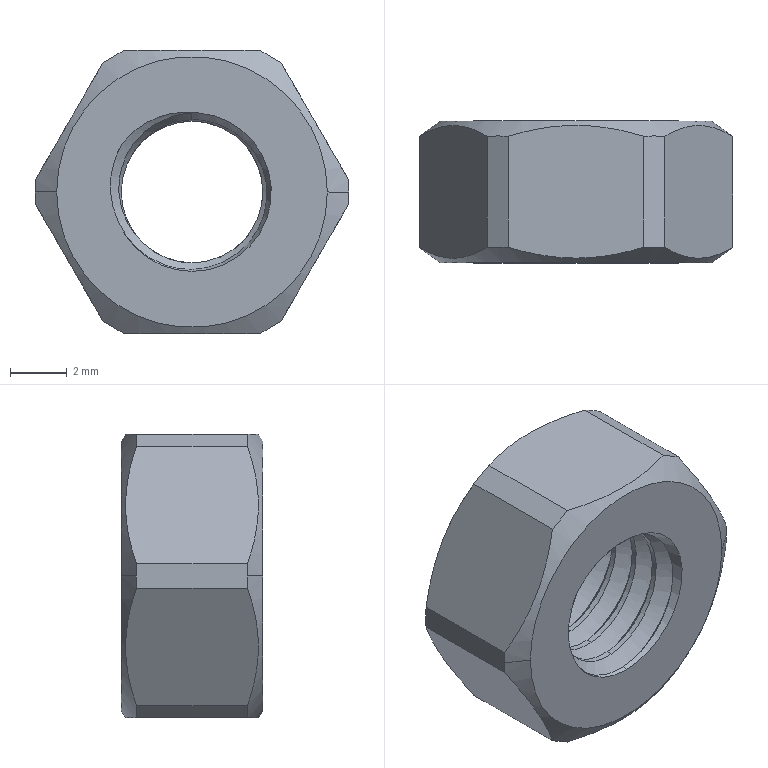Part | SolidWorks | features BaseBody 1, Chamfer 1 | 1 solid | 35 faces | box 11.05 x 5 x 10 mm | volume 308.187 mm3 | plane 14 | cone 10 | cylinder 9 | spline 2 | commonest cylinder face diameters 5 x9